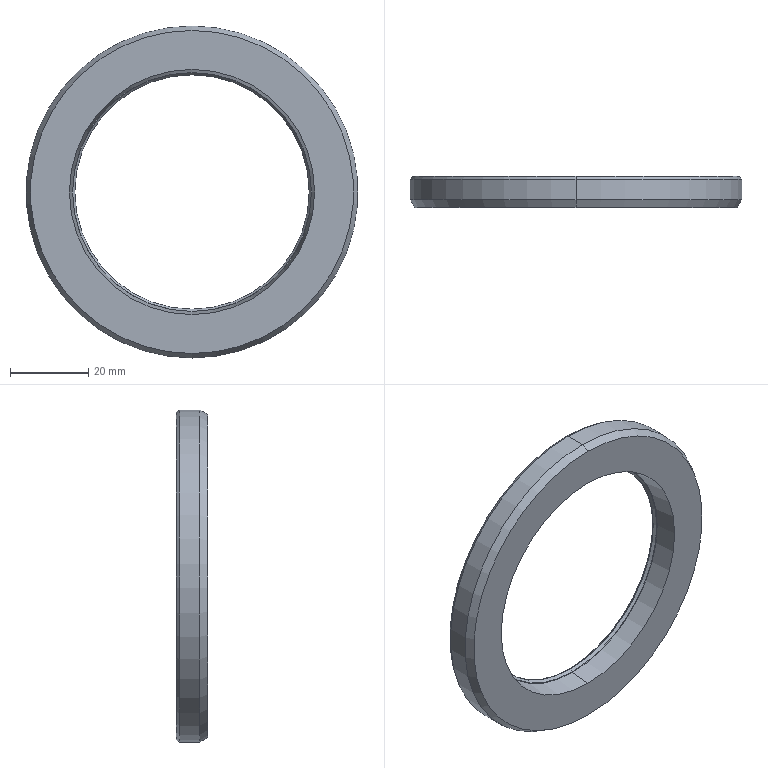Part | STEP file | Lip Seal GB/T13871.1-2007 Type B B58_B1 | 1 solid | 30 faces | box 85 x 8 x 85 mm | volume 12919 mm3 | cone 14 | torus 8 | cylinder 4 | plane 4 | commonest cylinder face diameters 67.143 x2 85 x2